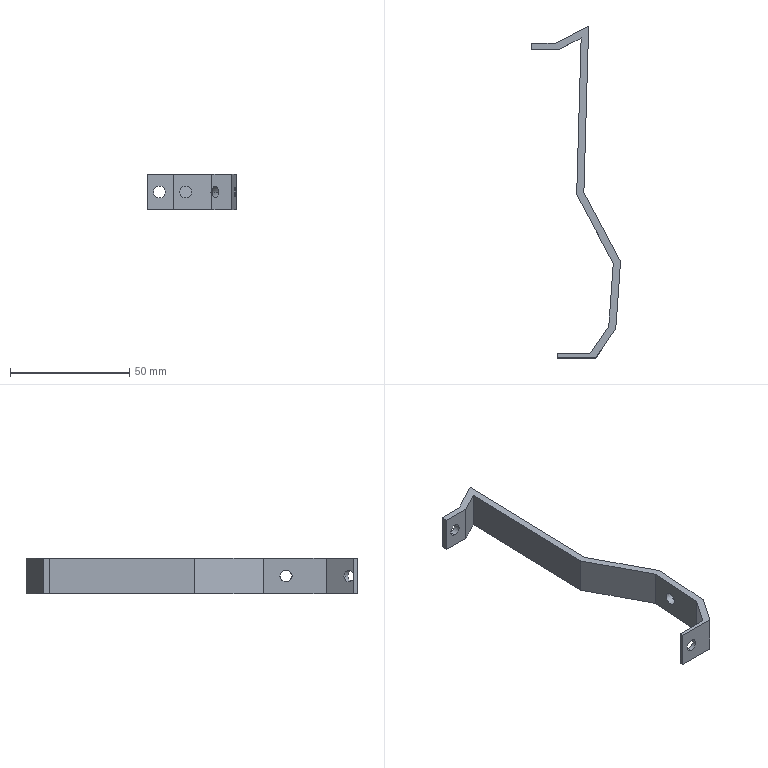Part | SolidWorks | features ICE 4, Extrusion 1, RevCut 1 | 1 solid | 26 faces | box 37.394 x 139.343 x 15 mm | volume 7600 mm3 | plane 18 | torus 4 | cylinder 4 | commonest cylinder face diameters 5 x4
STEP:
#1=CARTESIAN_POINT('',(17.078,-131.945,0.));
#2=VERTEX_POINT('',#1);
#3=CARTESIAN_POINT('',(19.895,-127.783,0.));
#4=VERTEX_POINT('',#3);
#5=CARTESIAN_POINT('',(17.078,-131.945,0.));
#6=CARTESIAN_POINT('',(17.078,-131.945,0.1641));
#7=CARTESIAN_POINT('',(17.087,-131.932,0.3266));
#8=CARTESIAN_POINT('',(17.123,-131.879,0.6485));
#9=CARTESIAN_POINT('',(17.15,-131.838,0.8079));
#10=CARTESIAN_POINT('',(17.256,-131.682,1.26));
#11=CARTESIAN_POINT('',(17.361,-131.527,1.54));
#12=CARTESIAN_POINT('',(17.556,-131.239,1.885));
#13=CARTESIAN_POINT('',(17.628,-131.132,1.99));
#14=CARTESIAN_POINT('',(17.782,-130.905,2.172));
#15=CARTESIAN_POINT('',(17.863,-130.785,2.248));
#16=CARTESIAN_POINT('',(18.033,-130.535,2.373));
#17=CARTESIAN_POINT('',(18.122,-130.402,2.421));
#18=CARTESIAN_POINT('',(18.302,-130.136,2.484));
#19=CARTESIAN_POINT('',(18.393,-130.002,2.5));
#20=CARTESIAN_POINT('',(18.578,-129.729,2.5));
#21=CARTESIAN_POINT('',(18.67,-129.592,2.484));
#22=CARTESIAN_POINT('',(18.85,-129.327,2.42));
#23=CARTESIAN_POINT('',(18.938,-129.196,2.373));
#24=CARTESIAN_POINT('',(19.11,-128.943,2.247));
#25=CARTESIAN_POINT('',(19.19,-128.824,2.17));
#26=CARTESIAN_POINT('',(19.343,-128.598,1.99));
#27=CARTESIAN_POINT('',(19.416,-128.491,1.885));
#28=CARTESIAN_POINT('',(19.546,-128.298,1.653));
#29=CARTESIAN_POINT('',(19.605,-128.212,1.528));
#30=CARTESIAN_POINT('',(19.707,-128.06,1.256));
#31=CARTESIAN_POINT('',(19.752,-127.994,1.109));
#32=CARTESIAN_POINT('',(19.858,-127.838,0.6566));
#33=CARTESIAN_POINT('',(19.895,-127.783,0.3266));
#34=CARTESIAN_POINT('',(19.895,-127.783,0.));
#35=B_SPLINE_CURVE_WITH_KNOTS('',3,(#5,#6,#7,#8,#9,#10,#11,#12,#13,#14,#15,#16,#17,#18,#19,#20,#21,#22,#23,#24,#25,#26,#27,#28,#29,#30,#31,#32,#33,#34),.UNSPECIFIED.,.F.,.F.,(4,2,2,2,2,2,2,2,2,2,2,2,2,2,4),(0.001854,0.002344,0.002834,0.003814,0.004304,0.004794,0.005284,0.005774,0.006263,0.006753,0.007243,0.007733,0.008223,0.008713,0.009693),.UNSPECIFIED.);
#36=EDGE_CURVE('',#2,#4,#35,.T.);
#37=ORIENTED_EDGE('',*,*,#36,.F.);
#38=CARTESIAN_POINT('',(14.593,-130.264,0.));
#39=VERTEX_POINT('',#38);
#40=CARTESIAN_POINT('',(25.607,-116.664,0.));
#41=DIRECTION('',(0.,0.,-1.));
#42=DIRECTION('',(-1.,0.,0.));
#43=AXIS2_PLACEMENT_3D('',#40,#41,#42);
#44=CIRCLE('',#43,17.5);
#45=EDGE_CURVE('',#2,#39,#44,.T.);
#46=ORIENTED_EDGE('',*,*,#45,.T.);
#47=CARTESIAN_POINT('',(17.41,-126.101,0.));
#48=VERTEX_POINT('',#47);
#49=CARTESIAN_POINT('',(17.41,-126.101,0.));
#50=CARTESIAN_POINT('',(17.41,-126.101,0.1645));
#51=CARTESIAN_POINT('',(17.401,-126.115,0.3271));
#52=CARTESIAN_POINT('',(17.365,-126.168,0.6482));
#53=CARTESIAN_POINT('',(17.338,-126.209,0.8078));
#54=CARTESIAN_POINT('',(17.267,-126.313,1.11));
#55=CARTESIAN_POINT('',(17.223,-126.377,1.254));
#56=CARTESIAN_POINT('',(17.12,-126.53,1.527));
#57=CARTESIAN_POINT('',(17.061,-126.617,1.654));
#58=CARTESIAN_POINT('',(16.866,-126.905,1.999));
#59=CARTESIAN_POINT('',(16.709,-127.138,2.185));
#60=CARTESIAN_POINT('',(16.455,-127.513,2.372));
#61=CARTESIAN_POINT('',(16.365,-127.645,2.42));
#62=CARTESIAN_POINT('',(16.185,-127.912,2.484));
#63=CARTESIAN_POINT('',(16.094,-128.046,2.5));
#64=CARTESIAN_POINT('',(15.91,-128.318,2.5));
#65=CARTESIAN_POINT('',(15.817,-128.456,2.484));
#66=CARTESIAN_POINT('',(15.637,-128.721,2.421));
#67=CARTESIAN_POINT('',(15.55,-128.851,2.374));
#68=CARTESIAN_POINT('',(15.378,-129.104,2.248));
#69=CARTESIAN_POINT('',(15.297,-129.224,2.171));
#70=CARTESIAN_POINT('',(15.144,-129.45,1.991));
#71=CARTESIAN_POINT('',(15.072,-129.556,1.886));
#72=CARTESIAN_POINT('',(14.941,-129.75,1.654));
#73=CARTESIAN_POINT('',(14.883,-129.836,1.528));
#74=CARTESIAN_POINT('',(14.781,-129.987,1.257));
#75=CARTESIAN_POINT('',(14.736,-130.053,1.11));
#76=CARTESIAN_POINT('',(14.666,-130.157,0.8073));
#77=CARTESIAN_POINT('',(14.639,-130.197,0.6512));
#78=CARTESIAN_POINT('',(14.603,-130.25,0.3285));
#79=CARTESIAN_POINT('',(14.593,-130.264,0.1633));
#80=CARTESIAN_POINT('',(14.593,-130.264,0.));
#81=B_SPLINE_CURVE_WITH_KNOTS('',3,(#49,#50,#51,#52,#53,#54,#55,#56,#57,#58,#59,#60,#61,#62,#63,#64,#65,#66,#67,#68,#69,#70,#71,#72,#73,#74,#75,#76,#77,#78,#79,#80),.UNSPECIFIED.,.F.,.F.,(4,2,2,2,2,2,2,2,2,2,2,2,2,2,2,4),(0.006023,0.006513,0.007003,0.007492,0.007982,0.008962,0.009452,0.009942,0.01043,0.01092,0.01141,0.0119,0.01239,0.01288,0.01337,0.01386),.UNSPECIFIED.);
#82=EDGE_CURVE('',#48,#39,#81,.T.);
#83=ORIENTED_EDGE('',*,*,#82,.F.);
#84=CARTESIAN_POINT('',(25.607,-116.664,0.));
#85=DIRECTION('',(0.,0.,-1.));
#86=DIRECTION('',(-1.,0.,0.));
#87=AXIS2_PLACEMENT_3D('',#84,#85,#86);
#88=CIRCLE('',#87,12.5);
#89=EDGE_CURVE('',#4,#48,#88,.T.);
#90=ORIENTED_EDGE('',*,*,#89,.F.);
#91=EDGE_LOOP('',(#37,#46,#83,#90));
#92=FACE_OUTER_BOUND('',#91,.T.);
#93=CARTESIAN_POINT('',(25.607,-116.664,0.));
#94=DIRECTION('',(0.,0.,-1.));
#95=DIRECTION('',(-1.,0.,0.));
#96=AXIS2_PLACEMENT_3D('',#93,#94,#95);
#97=TOROIDAL_SURFACE('',#96,15.,2.5);
#98=ADVANCED_FACE('',(#92),#97,.F.);
#99=CARTESIAN_POINT('',(23.843,-99.253,0.));
#100=VERTEX_POINT('',#99);
#101=CARTESIAN_POINT('',(23.479,-104.347,0.));
#102=VERTEX_POINT('',#101);
#103=CARTESIAN_POINT('',(23.843,-99.253,0.));
#104=CARTESIAN_POINT('',(23.843,-99.253,0.1653));
#105=CARTESIAN_POINT('',(23.842,-99.27,0.3291));
#106=CARTESIAN_POINT('',(23.837,-99.336,0.6537));
#107=CARTESIAN_POINT('',(23.834,-99.386,0.8139));
#108=CARTESIAN_POINT('',(23.82,-99.578,1.269));
#109=CARTESIAN_POINT('',(23.806,-99.77,1.548));
#110=CARTESIAN_POINT('',(23.781,-100.124,1.893));
#111=CARTESIAN_POINT('',(23.772,-100.255,1.998));
#112=CARTESIAN_POINT('',(23.752,-100.532,2.178));
#113=CARTESIAN_POINT('',(23.742,-100.678,2.253));
#114=CARTESIAN_POINT('',(23.72,-100.984,2.376));
#115=CARTESIAN_POINT('',(23.708,-101.145,2.423));
#116=CARTESIAN_POINT('',(23.685,-101.468,2.485));
#117=CARTESIAN_POINT('',(23.673,-101.631,2.5));
#118=CARTESIAN_POINT('',(23.638,-102.13,2.499));
#119=CARTESIAN_POINT('',(23.614,-102.456,2.435));
#120=CARTESIAN_POINT('',(23.582,-102.917,2.249));
#121=CARTESIAN_POINT('',(23.571,-103.063,2.173));
#122=CARTESIAN_POINT('',(23.551,-103.339,1.994));
#123=CARTESIAN_POINT('',(23.542,-103.47,1.889));
#124=CARTESIAN_POINT('',(23.525,-103.707,1.66));
#125=CARTESIAN_POINT('',(23.517,-103.814,1.534));
#126=CARTESIAN_POINT('',(23.504,-104.002,1.263));
#127=CARTESIAN_POINT('',(23.498,-104.083,1.116));
#128=CARTESIAN_POINT('',(23.489,-104.213,0.813));
#129=CARTESIAN_POINT('',(23.485,-104.263,0.656));
#130=CARTESIAN_POINT('',(23.481,-104.33,0.33));
#131=CARTESIAN_POINT('',(23.479,-104.347,0.1646));
#132=CARTESIAN_POINT('',(23.479,-104.347,0.));
#133=B_SPLINE_CURVE_WITH_KNOTS('',3,(#103,#104,#105,#106,#107,#108,#109,#110,#111,#112,#113,#114,#115,#116,#117,#118,#119,#120,#121,#122,#123,#124,#125,#126,#127,#128,#129,#130,#131,#132),.UNSPECIFIED.,.F.,.F.,(4,2,2,2,2,2,2,2,2,2,2,2,2,2,4),(0.007039,0.007533,0.008027,0.009014,0.009508,0.01,0.0105,0.01099,0.01198,0.01247,0.01296,0.01346,0.01395,0.01445,0.01494),.UNSPECIFIED.);
#134=EDGE_CURVE('',#100,#102,#133,.T.);
#135=ORIENTED_EDGE('',*,*,#134,.F.);
#136=CARTESIAN_POINT('',(26.854,-99.209,0.));
#137=VERTEX_POINT('',#136);
#138=CARTESIAN_POINT('',(25.607,-116.664,0.));
#139=DIRECTION('',(0.,0.,-1.));
#140=DIRECTION('',(-1.,0.,0.));
#141=AXIS2_PLACEMENT_3D('',#138,#139,#140);
#142=CIRCLE('',#141,17.5);
#143=EDGE_CURVE('',#100,#137,#142,.T.);
#144=ORIENTED_EDGE('',*,*,#143,.T.);
#145=CARTESIAN_POINT('',(26.498,-104.196,0.));
#146=VERTEX_POINT('',#145);
#147=CARTESIAN_POINT('',(26.676,-101.702,0.));
#148=DIRECTION('',(-0.9975,0.07125,0.));
#149=DIRECTION('',(-0.07125,-0.9975,0.));
#150=AXIS2_PLACEMENT_3D('',#147,#148,#149);
#151=CIRCLE('',#150,2.5);
#152=EDGE_CURVE('',#146,#137,#151,.T.);
#153=ORIENTED_EDGE('',*,*,#152,.F.);
#154=CARTESIAN_POINT('',(25.607,-116.664,0.));
#155=DIRECTION('',(0.,0.,-1.));
#156=DIRECTION('',(-1.,0.,0.));
#157=AXIS2_PLACEMENT_3D('',#154,#155,#156);
#158=CIRCLE('',#157,12.5);
#159=EDGE_CURVE('',#102,#146,#158,.T.);
#160=ORIENTED_EDGE('',*,*,#159,.F.);
#161=EDGE_LOOP('',(#135,#144,#153,#160));
#162=FACE_OUTER_BOUND('',#161,.T.);
#163=CARTESIAN_POINT('',(25.607,-116.664,0.));
#164=DIRECTION('',(0.,0.,-1.));
#165=DIRECTION('',(-1.,0.,0.));
#166=AXIS2_PLACEMENT_3D('',#163,#164,#165);
#167=TOROIDAL_SURFACE('',#166,15.,2.5);
#168=ADVANCED_FACE('',(#162),#167,.F.);
#169=CARTESIAN_POINT('',(6.,-130.319,-2.5));
#170=VERTEX_POINT('',#169);
#171=CARTESIAN_POINT('',(6.,-130.319,2.5));
#172=VERTEX_POINT('',#171);
#173=CARTESIAN_POINT('',(6.,-130.319,0.));
#174=DIRECTION('',(0.,1.,0.));
#175=DIRECTION('',(0.,0.,1.));
#176=AXIS2_PLACEMENT_3D('',#173,#174,#175);
#177=CIRCLE('',#176,2.5);
#178=EDGE_CURVE('',#170,#172,#177,.T.);
#179=ORIENTED_EDGE('',*,*,#178,.T.);
#180=CARTESIAN_POINT('',(6.,-132.,2.5));
#181=VERTEX_POINT('',#180);
#182=CARTESIAN_POINT('',(6.,-122.,2.5));
#183=DIRECTION('',(0.,-1.,0.));
#184=VECTOR('',#183,1000.);
#185=LINE('',#182,#184);
#186=EDGE_CURVE('',#172,#181,#185,.T.);
#187=ORIENTED_EDGE('',*,*,#186,.T.);
#188=CARTESIAN_POINT('',(6.,-132.,-2.5));
#189=VERTEX_POINT('',#188);
#190=CARTESIAN_POINT('',(6.,-132.,0.));
#191=DIRECTION('',(0.,-1.,0.));
#192=DIRECTION('',(0.,0.,-1.));
#193=AXIS2_PLACEMENT_3D('',#190,#191,#192);
#194=CIRCLE('',#193,2.5);
#195=EDGE_CURVE('',#181,#189,#194,.T.);
#196=ORIENTED_EDGE('',*,*,#195,.T.);
#197=CARTESIAN_POINT('',(6.,-122.,-2.5));
#198=DIRECTION('',(0.,-1.,0.));
#199=VECTOR('',#198,1000.);
#200=LINE('',#197,#199);
#201=EDGE_CURVE('',#170,#189,#200,.T.);
#202=ORIENTED_EDGE('',*,*,#201,.F.);
#203=EDGE_LOOP('',(#179,#187,#196,#202));
#204=FACE_OUTER_BOUND('',#203,.T.);
#205=CARTESIAN_POINT('',(6.,-122.,0.));
#206=DIRECTION('',(0.,-1.,0.));
#207=DIRECTION('',(0.,0.,-1.));
#208=AXIS2_PLACEMENT_3D('',#205,#206,#207);
#209=CYLINDRICAL_SURFACE('',#208,2.5);
#210=ADVANCED_FACE('',(#204),#209,.F.);
#211=CARTESIAN_POINT('',(-5.,-2.657,2.5));
#212=VERTEX_POINT('',#211);
#213=CARTESIAN_POINT('',(-5.,-2.657,-2.5));
#214=VERTEX_POINT('',#213);
#215=CARTESIAN_POINT('',(-5.,-2.657,0.));
#216=DIRECTION('',(0.,-1.,0.));
#217=DIRECTION('',(0.,0.,-1.));
#218=AXIS2_PLACEMENT_3D('',#215,#216,#217);
#219=CIRCLE('',#218,2.5);
#220=EDGE_CURVE('',#212,#214,#219,.T.);
#221=ORIENTED_EDGE('',*,*,#220,.T.);
#222=CARTESIAN_POINT('',(-5.,0.,-2.5));
#223=VERTEX_POINT('',#222);
#224=CARTESIAN_POINT('',(-5.,-5.,-2.5));
#225=DIRECTION('',(0.,1.,0.));
#226=VECTOR('',#225,1000.);
#227=LINE('',#224,#226);
#228=EDGE_CURVE('',#214,#223,#227,.T.);
#229=ORIENTED_EDGE('',*,*,#228,.T.);
#230=CARTESIAN_POINT('',(-5.,0.,2.5));
#231=VERTEX_POINT('',#230);
#232=CARTESIAN_POINT('',(-5.,0.,0.));
#233=DIRECTION('',(0.,1.,0.));
#234=DIRECTION('',(0.,0.,1.));
#235=AXIS2_PLACEMENT_3D('',#232,#233,#234);
#236=CIRCLE('',#235,2.5);
#237=EDGE_CURVE('',#223,#231,#236,.T.);
#238=ORIENTED_EDGE('',*,*,#237,.T.);
#239=CARTESIAN_POINT('',(-5.,-5.,2.5));
#240=DIRECTION('',(0.,1.,0.));
#241=VECTOR('',#240,1000.);
#242=LINE('',#239,#241);
#243=EDGE_CURVE('',#212,#231,#242,.T.);
#244=ORIENTED_EDGE('',*,*,#243,.F.);
#245=EDGE_LOOP('',(#221,#229,#238,#244));
#246=FACE_OUTER_BOUND('',#245,.T.);
#247=CARTESIAN_POINT('',(-5.,-5.,0.));
#248=DIRECTION('',(0.,1.,0.));
#249=DIRECTION('',(0.,0.,1.));
#250=AXIS2_PLACEMENT_3D('',#247,#248,#249);
#251=CYLINDRICAL_SURFACE('',#250,2.5);
#252=ADVANCED_FACE('',(#246),#251,.F.);
#253=CARTESIAN_POINT('',(1.394,-2.657,-7.5));
#254=VERTEX_POINT('',#253);
#255=CARTESIAN_POINT('',(10.855,2.306,-7.5));
#256=VERTEX_POINT('',#255);
#257=CARTESIAN_POINT('',(1.394,-2.657,-7.5));
#258=DIRECTION('',(0.8856,0.4645,0.));
#259=VECTOR('',#258,1000.);
#260=LINE('',#257,#259);
#261=EDGE_CURVE('',#254,#256,#260,.T.);
#262=ORIENTED_EDGE('',*,*,#261,.T.);
#263=CARTESIAN_POINT('',(10.855,2.306,7.5));
#264=VERTEX_POINT('',#263);
#265=CARTESIAN_POINT('',(10.855,2.306,7.5));
#266=DIRECTION('',(0.,0.,-1.));
#267=VECTOR('',#266,1000.);
#268=LINE('',#265,#267);
#269=EDGE_CURVE('',#264,#256,#268,.T.);
#270=ORIENTED_EDGE('',*,*,#269,.F.);
#271=CARTESIAN_POINT('',(1.394,-2.657,7.5));
#272=VERTEX_POINT('',#271);
#273=CARTESIAN_POINT('',(1.394,-2.657,7.5));
#274=DIRECTION('',(0.8856,0.4645,0.));
#275=VECTOR('',#274,1000.);
#276=LINE('',#273,#275);
#277=EDGE_CURVE('',#272,#264,#276,.T.);
#278=ORIENTED_EDGE('',*,*,#277,.F.);
#279=CARTESIAN_POINT('',(1.394,-2.657,7.5));
#280=DIRECTION('',(0.,0.,-1.));
#281=VECTOR('',#280,1000.);
#282=LINE('',#279,#281);
#283=EDGE_CURVE('',#272,#254,#282,.T.);
#284=ORIENTED_EDGE('',*,*,#283,.T.);
#285=EDGE_LOOP('',(#262,#270,#278,#284));
#286=FACE_OUTER_BOUND('',#285,.T.);
#287=CARTESIAN_POINT('',(1.394,-2.657,7.5));
#288=DIRECTION('',(-0.4645,0.8856,0.));
#289=DIRECTION('',(-0.8856,-0.4645,0.));
#290=AXIS2_PLACEMENT_3D('',#287,#288,#289);
#291=PLANE('',#290);
#292=ADVANCED_FACE('',(#286),#291,.F.);
#293=CARTESIAN_POINT('',(8.979,-63.363,-7.5));
#294=VERTEX_POINT('',#293);
#295=CARTESIAN_POINT('',(10.855,2.306,-7.5));
#296=DIRECTION('',(-0.02856,-0.9996,0.));
#297=VECTOR('',#296,1000.);
#298=LINE('',#295,#297);
#299=EDGE_CURVE('',#256,#294,#298,.T.);
#300=ORIENTED_EDGE('',*,*,#299,.T.);
#301=CARTESIAN_POINT('',(8.979,-63.363,7.5));
#302=VERTEX_POINT('',#301);
#303=CARTESIAN_POINT('',(8.979,-63.363,7.5));
#304=DIRECTION('',(0.,0.,-1.));
#305=VECTOR('',#304,1000.);
#306=LINE('',#303,#305);
#307=EDGE_CURVE('',#302,#294,#306,.T.);
#308=ORIENTED_EDGE('',*,*,#307,.F.);
#309=CARTESIAN_POINT('',(10.855,2.306,7.5));
#310=DIRECTION('',(-0.02856,-0.9996,0.));
#311=VECTOR('',#310,1000.);
#312=LINE('',#309,#311);
#313=EDGE_CURVE('',#264,#302,#312,.T.);
#314=ORIENTED_EDGE('',*,*,#313,.F.);
#315=ORIENTED_EDGE('',*,*,#269,.T.);
#316=EDGE_LOOP('',(#300,#308,#314,#315));
#317=FACE_OUTER_BOUND('',#316,.T.);
#318=CARTESIAN_POINT('',(10.855,2.306,7.5));
#319=DIRECTION('',(0.9996,-0.02856,0.));
#320=DIRECTION('',(0.02856,0.9996,0.));
#321=AXIS2_PLACEMENT_3D('',#318,#319,#320);
#322=PLANE('',#321);
#323=ADVANCED_FACE('',(#317),#322,.F.);
#324=CARTESIAN_POINT('',(24.34,-92.302,-7.5));
#325=VERTEX_POINT('',#324);
#326=CARTESIAN_POINT('',(8.979,-63.363,-7.5));
#327=DIRECTION('',(0.4689,-0.8833,0.));
#328=VECTOR('',#327,1000.);
#329=LINE('',#326,#328);
#330=EDGE_CURVE('',#294,#325,#329,.T.);
#331=ORIENTED_EDGE('',*,*,#330,.T.);
#332=CARTESIAN_POINT('',(24.34,-92.302,7.5));
#333=VERTEX_POINT('',#332);
#334=CARTESIAN_POINT('',(24.34,-92.302,7.5));
#335=DIRECTION('',(0.,0.,-1.));
#336=VECTOR('',#335,1000.);
#337=LINE('',#334,#336);
#338=EDGE_CURVE('',#333,#325,#337,.T.);
#339=ORIENTED_EDGE('',*,*,#338,.F.);
#340=CARTESIAN_POINT('',(8.979,-63.363,7.5));
#341=DIRECTION('',(0.4689,-0.8833,0.));
#342=VECTOR('',#341,1000.);
#343=LINE('',#340,#342);
#344=EDGE_CURVE('',#302,#333,#343,.T.);
#345=ORIENTED_EDGE('',*,*,#344,.F.);
#346=ORIENTED_EDGE('',*,*,#307,.T.);
#347=EDGE_LOOP('',(#331,#339,#345,#346));
#348=FACE_OUTER_BOUND('',#347,.T.);
#349=CARTESIAN_POINT('',(8.979,-63.363,7.5));
#350=DIRECTION('',(0.8833,0.4689,0.));
#351=DIRECTION('',(-0.4689,0.8833,0.));
#352=AXIS2_PLACEMENT_3D('',#349,#350,#351);
#353=PLANE('',#352);
#354=ADVANCED_FACE('',(#348),#353,.F.);
#355=CARTESIAN_POINT('',(23.479,-104.347,0.));
#356=CARTESIAN_POINT('',(23.479,-104.347,-0.329));
#357=CARTESIAN_POINT('',(23.484,-104.277,-0.6643));
#358=CARTESIAN_POINT('',(23.498,-104.081,-1.12));
#359=CARTESIAN_POINT('',(23.504,-104.001,-1.264));
#360=CARTESIAN_POINT('',(23.518,-103.813,-1.535));
#361=CARTESIAN_POINT('',(23.525,-103.704,-1.663));
#362=CARTESIAN_POINT('',(23.542,-103.467,-1.892));
#363=CARTESIAN_POINT('',(23.551,-103.339,-1.994));
#364=CARTESIAN_POINT('',(23.571,-103.06,-2.174));
#365=CARTESIAN_POINT('',(23.582,-102.913,-2.251));
#366=CARTESIAN_POINT('',(23.614,-102.456,-2.435));
#367=CARTESIAN_POINT('',(23.638,-102.124,-2.499));
#368=CARTESIAN_POINT('',(23.673,-101.632,-2.5));
#369=CARTESIAN_POINT('',(23.685,-101.465,-2.485));
#370=CARTESIAN_POINT('',(23.708,-101.141,-2.422));
#371=CARTESIAN_POINT('',(23.72,-100.984,-2.376));
#372=CARTESIAN_POINT('',(23.741,-100.678,-2.253));
#373=CARTESIAN_POINT('',(23.752,-100.529,-2.176));
#374=CARTESIAN_POINT('',(23.772,-100.253,-1.997));
#375=CARTESIAN_POINT('',(23.781,-100.125,-1.894));
#376=CARTESIAN_POINT('',(23.806,-99.769,-1.547));
#377=CARTESIAN_POINT('',(23.82,-99.58,-1.272));
#378=CARTESIAN_POINT('',(23.834,-99.385,-0.8125));
#379=CARTESIAN_POINT('',(23.837,-99.336,-0.6552));
#380=CARTESIAN_POINT('',(23.842,-99.27,-0.3325));
#381=CARTESIAN_POINT('',(23.843,-99.253,-0.1652));
#382=CARTESIAN_POINT('',(23.843,-99.253,0.));
#383=B_SPLINE_CURVE_WITH_KNOTS('',3,(#355,#356,#357,#358,#359,#360,#361,#362,#363,#364,#365,#366,#367,#368,#369,#370,#371,#372,#373,#374,#375,#376,#377,#378,#379,#380,#381,#382),.UNSPECIFIED.,.F.,.F.,(4,2,2,2,2,2,2,2,2,2,2,2,2,4),(0.01494,0.01593,0.01642,0.01691,0.01741,0.0179,0.01889,0.01938,0.01987,0.02037,0.02086,0.02185,0.02234,0.02283),.UNSPECIFIED.);
#384=EDGE_CURVE('',#102,#100,#383,.T.);
#385=ORIENTED_EDGE('',*,*,#384,.T.);
#386=ORIENTED_EDGE('',*,*,#134,.T.);
#387=EDGE_LOOP('',(#385,#386));
#388=FACE_BOUND('',#387,.T.);
#389=CARTESIAN_POINT('',(22.458,-118.641,-7.5));
#390=VERTEX_POINT('',#389);
#391=CARTESIAN_POINT('',(24.34,-92.302,-7.5));
#392=DIRECTION('',(-0.07125,-0.9975,0.));
#393=VECTOR('',#392,1000.);
#394=LINE('',#391,#393);
#395=EDGE_CURVE('',#325,#390,#394,.T.);
#396=ORIENTED_EDGE('',*,*,#395,.T.);
#397=CARTESIAN_POINT('',(22.458,-118.641,7.5));
#398=VERTEX_POINT('',#397);
#399=CARTESIAN_POINT('',(22.458,-118.641,7.5));
#400=DIRECTION('',(0.,0.,-1.));
#401=VECTOR('',#400,1000.);
#402=LINE('',#399,#401);
#403=EDGE_CURVE('',#398,#390,#402,.T.);
#404=ORIENTED_EDGE('',*,*,#403,.F.);
#405=CARTESIAN_POINT('',(24.34,-92.302,7.5));
#406=DIRECTION('',(-0.07125,-0.9975,0.));
#407=VECTOR('',#406,1000.);
#408=LINE('',#405,#407);
#409=EDGE_CURVE('',#333,#398,#408,.T.);
#410=ORIENTED_EDGE('',*,*,#409,.F.);
#411=ORIENTED_EDGE('',*,*,#338,.T.);
#412=EDGE_LOOP('',(#396,#404,#410,#411));
#413=FACE_OUTER_BOUND('',#412,.T.);
#414=CARTESIAN_POINT('',(24.34,-92.302,7.5));
#415=DIRECTION('',(0.9975,-0.07125,0.));
#416=DIRECTION('',(0.07125,0.9975,0.));
#417=AXIS2_PLACEMENT_3D('',#414,#415,#416);
#418=PLANE('',#417);
#419=ADVANCED_FACE('',(#388,#413),#418,.F.);
#420=ORIENTED_EDGE('',*,*,#82,.T.);
#421=CARTESIAN_POINT('',(14.593,-130.264,0.));
#422=CARTESIAN_POINT('',(14.593,-130.264,-0.3265));
#423=CARTESIAN_POINT('',(14.63,-130.209,-0.6563));
#424=CARTESIAN_POINT('',(14.771,-130.001,-1.26));
#425=CARTESIAN_POINT('',(14.877,-129.844,-1.541));
#426=CARTESIAN_POINT('',(15.073,-129.555,-1.888));
#427=CARTESIAN_POINT('',(15.144,-129.45,-1.991));
#428=CARTESIAN_POINT('',(15.297,-129.224,-2.172));
#429=CARTESIAN_POINT('',(15.38,-129.102,-2.25));
#430=CARTESIAN_POINT('',(15.55,-128.851,-2.374));
#431=CARTESIAN_POINT('',(15.637,-128.721,-2.421));
#432=CARTESIAN_POINT('',(15.819,-128.454,-2.484));
#433=CARTESIAN_POINT('',(15.911,-128.317,-2.5));
#434=CARTESIAN_POINT('',(16.094,-128.047,-2.5));
#435=CARTESIAN_POINT('',(16.186,-127.911,-2.484));
#436=CARTESIAN_POINT('',(16.367,-127.643,-2.42));
#437=CARTESIAN_POINT('',(16.455,-127.514,-2.372));
#438=CARTESIAN_POINT('',(16.624,-127.263,-2.248));
#439=CARTESIAN_POINT('',(16.706,-127.141,-2.17));
#440=CARTESIAN_POINT('',(16.86,-126.915,-1.988));
#441=CARTESIAN_POINT('',(16.93,-126.81,-1.885));
#442=CARTESIAN_POINT('',(17.061,-126.617,-1.654));
#443=CARTESIAN_POINT('',(17.121,-126.529,-1.526));
#444=CARTESIAN_POINT('',(17.223,-126.378,-1.255));
#445=CARTESIAN_POINT('',(17.266,-126.314,-1.112));
#446=CARTESIAN_POINT('',(17.338,-126.208,-0.8067));
#447=CARTESIAN_POINT('',(17.365,-126.168,-0.6496));
#448=CARTESIAN_POINT('',(17.401,-126.115,-0.3296));
#449=CARTESIAN_POINT('',(17.41,-126.101,-0.1645));
#450=CARTESIAN_POINT('',(17.41,-126.101,0.));
#451=B_SPLINE_CURVE_WITH_KNOTS('',3,(#421,#422,#423,#424,#425,#426,#427,#428,#429,#430,#431,#432,#433,#434,#435,#436,#437,#438,#439,#440,#441,#442,#443,#444,#445,#446,#447,#448,#449,#450),.UNSPECIFIED.,.F.,.F.,(4,2,2,2,2,2,2,2,2,2,2,2,2,2,4),(0.01386,0.01484,0.01582,0.01631,0.0168,0.01729,0.01778,0.01827,0.01876,0.01925,0.01973,0.02022,0.02071,0.0212,0.02169),.UNSPECIFIED.);
#452=EDGE_CURVE('',#39,#48,#451,.T.);
#453=ORIENTED_EDGE('',*,*,#452,.T.);
#454=EDGE_LOOP('',(#420,#453));
#455=FACE_BOUND('',#454,.T.);
#456=CARTESIAN_POINT('',(14.556,-130.319,-7.5));
#457=VERTEX_POINT('',#456);
#458=CARTESIAN_POINT('',(22.458,-118.641,-7.5));
#459=DIRECTION('',(-0.5604,-0.8282,0.));
#460=VECTOR('',#459,1000.);
#461=LINE('',#458,#460);
#462=EDGE_CURVE('',#390,#457,#461,.T.);
#463=ORIENTED_EDGE('',*,*,#462,.T.);
#464=CARTESIAN_POINT('',(14.556,-130.319,7.5));
#465=VERTEX_POINT('',#464);
#466=CARTESIAN_POINT('',(14.556,-130.319,7.5));
#467=DIRECTION('',(0.,0.,-1.));
#468=VECTOR('',#467,1000.);
#469=LINE('',#466,#468);
#470=EDGE_CURVE('',#465,#457,#469,.T.);
#471=ORIENTED_EDGE('',*,*,#470,.F.);
#472=CARTESIAN_POINT('',(22.458,-118.641,7.5));
#473=DIRECTION('',(-0.5604,-0.8282,0.));
#474=VECTOR('',#473,1000.);
#475=LINE('',#472,#474);
#476=EDGE_CURVE('',#398,#465,#475,.T.);
#477=ORIENTED_EDGE('',*,*,#476,.F.);
#478=ORIENTED_EDGE('',*,*,#403,.T.);
#479=EDGE_LOOP('',(#463,#471,#477,#478));
#480=FACE_OUTER_BOUND('',#479,.T.);
#481=CARTESIAN_POINT('',(22.458,-118.641,7.5));
#482=DIRECTION('',(0.8282,-0.5604,0.));
#483=DIRECTION('',(0.5604,0.8282,0.));
#484=AXIS2_PLACEMENT_3D('',#481,#482,#483);
#485=PLANE('',#484);
#486=ADVANCED_FACE('',(#455,#480),#485,.F.);
#487=CARTESIAN_POINT('',(19.895,-127.783,0.));
#488=CARTESIAN_POINT('',(19.895,-127.783,-0.1632));
#489=CARTESIAN_POINT('',(19.886,-127.796,-0.328));
#490=CARTESIAN_POINT('',(19.849,-127.85,-0.6508));
#491=CARTESIAN_POINT('',(19.822,-127.89,-0.8069));
#492=CARTESIAN_POINT('',(19.752,-127.994,-1.109));
#493=CARTESIAN_POINT('',(19.707,-128.06,-1.256));
#494=CARTESIAN_POINT('',(19.605,-128.211,-1.527));
#495=CARTESIAN_POINT('',(19.547,-128.297,-1.653));
#496=CARTESIAN_POINT('',(19.416,-128.491,-1.884));
#497=CARTESIAN_POINT('',(19.344,-128.597,-1.989));
#498=CARTESIAN_POINT('',(19.191,-128.823,-2.17));
#499=CARTESIAN_POINT('',(19.11,-128.943,-2.247));
#500=CARTESIAN_POINT('',(18.939,-129.196,-2.373));
#501=CARTESIAN_POINT('',(18.851,-129.325,-2.42));
#502=CARTESIAN_POINT('',(18.671,-129.591,-2.483));
#503=CARTESIAN_POINT('',(18.578,-129.728,-2.5));
#504=CARTESIAN_POINT('',(18.395,-130.,-2.5));
#505=CARTESIAN_POINT('',(18.304,-130.134,-2.484));
#506=CARTESIAN_POINT('',(18.123,-130.4,-2.422));
#507=CARTESIAN_POINT('',(18.034,-130.533,-2.374));
#508=CARTESIAN_POINT('',(17.78,-130.908,-2.188));
#509=CARTESIAN_POINT('',(17.623,-131.14,-2.003));
#510=CARTESIAN_POINT('',(17.361,-131.528,-1.538));
#511=CARTESIAN_POINT('',(17.257,-131.681,-1.264));
#512=CARTESIAN_POINT('',(17.15,-131.839,-0.8064));
#513=CARTESIAN_POINT('',(17.123,-131.878,-0.6501));
#514=CARTESIAN_POINT('',(17.087,-131.931,-0.3298));
#515=CARTESIAN_POINT('',(17.078,-131.945,-0.164));
#516=CARTESIAN_POINT('',(17.078,-131.945,0.));
#517=B_SPLINE_CURVE_WITH_KNOTS('',3,(#487,#488,#489,#490,#491,#492,#493,#494,#495,#496,#497,#498,#499,#500,#501,#502,#503,#504,#505,#506,#507,#508,#509,#510,#511,#512,#513,#514,#515,#516),.UNSPECIFIED.,.F.,.F.,(4,2,2,2,2,2,2,2,2,2,2,2,2,2,4),(0.009693,0.01018,0.01067,0.01116,0.01165,0.01214,0.01263,0.01312,0.01361,0.0141,0.01459,0.01557,0.01655,0.01704,0.01753),.UNSPECIFIED.);
#518=EDGE_CURVE('',#4,#2,#517,.T.);
#519=ORIENTED_EDGE('',*,*,#518,.T.);
#520=ORIENTED_EDGE('',*,*,#36,.T.);
#521=EDGE_LOOP('',(#519,#520));
#522=FACE_BOUND('',#521,.T.);
#523=CARTESIAN_POINT('',(17.041,-132.,-7.5));
#524=VERTEX_POINT('',#523);
#525=CARTESIAN_POINT('',(25.394,-119.657,-7.5));
#526=VERTEX_POINT('',#525);
#527=CARTESIAN_POINT('',(25.394,-119.657,-7.5));
#528=DIRECTION('',(0.5604,0.8282,0.));
#529=VECTOR('',#528,1000.);
#530=LINE('',#527,#529);
#531=EDGE_CURVE('',#524,#526,#530,.T.);
#532=ORIENTED_EDGE('',*,*,#531,.T.);
#533=CARTESIAN_POINT('',(25.394,-119.657,7.5));
#534=VERTEX_POINT('',#533);
#535=CARTESIAN_POINT('',(25.394,-119.657,7.5));
#536=DIRECTION('',(0.,0.,-1.));
#537=VECTOR('',#536,1000.);
#538=LINE('',#535,#537);
#539=EDGE_CURVE('',#534,#526,#538,.T.);
#540=ORIENTED_EDGE('',*,*,#539,.F.);
#541=CARTESIAN_POINT('',(17.041,-132.,7.5));
#542=VERTEX_POINT('',#541);
#543=CARTESIAN_POINT('',(25.394,-119.657,7.5));
#544=DIRECTION('',(0.5604,0.8282,0.));
#545=VECTOR('',#544,1000.);
#546=LINE('',#543,#545);
#547=EDGE_CURVE('',#542,#534,#546,.T.);
#548=ORIENTED_EDGE('',*,*,#547,.F.);
#549=CARTESIAN_POINT('',(17.041,-132.,7.5));
#550=DIRECTION('',(0.,0.,-1.));
#551=VECTOR('',#550,1000.);
#552=LINE('',#549,#551);
#553=EDGE_CURVE('',#542,#524,#552,.T.);
#554=ORIENTED_EDGE('',*,*,#553,.T.);
#555=EDGE_LOOP('',(#532,#540,#548,#554));
#556=FACE_OUTER_BOUND('',#555,.T.);
#557=CARTESIAN_POINT('',(25.394,-119.657,7.5));
#558=DIRECTION('',(-0.8282,0.5604,0.));
#559=DIRECTION('',(-0.5604,-0.8282,0.));
#560=AXIS2_PLACEMENT_3D('',#557,#558,#559);
#561=PLANE('',#560);
#562=ADVANCED_FACE('',(#522,#556),#561,.F.);
#563=ORIENTED_EDGE('',*,*,#152,.T.);
#564=CARTESIAN_POINT('',(26.676,-101.702,0.));
#565=DIRECTION('',(-0.9975,0.07125,0.));
#566=DIRECTION('',(-0.07125,-0.9975,0.));
#567=AXIS2_PLACEMENT_3D('',#564,#565,#566);
#568=CIRCLE('',#567,2.5);
#569=EDGE_CURVE('',#137,#146,#568,.T.);
#570=ORIENTED_EDGE('',*,*,#569,.T.);
#571=EDGE_LOOP('',(#563,#570));
#572=FACE_BOUND('',#571,.T.);
#573=CARTESIAN_POINT('',(27.394,-91.657,-7.5));
#574=VERTEX_POINT('',#573);
#575=CARTESIAN_POINT('',(27.394,-91.657,-7.5));
#576=DIRECTION('',(0.07125,0.9975,0.));
#577=VECTOR('',#576,1000.);
#578=LINE('',#575,#577);
#579=EDGE_CURVE('',#526,#574,#578,.T.);
#580=ORIENTED_EDGE('',*,*,#579,.T.);
#581=CARTESIAN_POINT('',(27.394,-91.657,7.5));
#582=VERTEX_POINT('',#581);
#583=CARTESIAN_POINT('',(27.394,-91.657,7.5));
#584=DIRECTION('',(0.,0.,-1.));
#585=VECTOR('',#584,1000.);
#586=LINE('',#583,#585);
#587=EDGE_CURVE('',#582,#574,#586,.T.);
#588=ORIENTED_EDGE('',*,*,#587,.F.);
#589=CARTESIAN_POINT('',(27.394,-91.657,7.5));
#590=DIRECTION('',(0.07125,0.9975,0.));
#591=VECTOR('',#590,1000.);
#592=LINE('',#589,#591);
#593=EDGE_CURVE('',#534,#582,#592,.T.);
#594=ORIENTED_EDGE('',*,*,#593,.F.);
#595=ORIENTED_EDGE('',*,*,#539,.T.);
#596=EDGE_LOOP('',(#580,#588,#594,#595));
#597=FACE_OUTER_BOUND('',#596,.T.);
#598=CARTESIAN_POINT('',(27.394,-91.657,7.5));
#599=DIRECTION('',(-0.9975,0.07125,0.));
#600=DIRECTION('',(-0.07125,-0.9975,0.));
#601=AXIS2_PLACEMENT_3D('',#598,#599,#600);
#602=PLANE('',#601);
#603=ADVANCED_FACE('',(#572,#597),#602,.F.);
#604=CARTESIAN_POINT('',(12.,-62.657,-7.5));
#605=VERTEX_POINT('',#604);
#606=CARTESIAN_POINT('',(12.,-62.657,-7.5));
#607=DIRECTION('',(-0.4689,0.8833,0.));
#608=VECTOR('',#607,1000.);
#609=LINE('',#606,#608);
#610=EDGE_CURVE('',#574,#605,#609,.T.);
#611=ORIENTED_EDGE('',*,*,#610,.T.);
#612=CARTESIAN_POINT('',(12.,-62.657,7.5));
#613=VERTEX_POINT('',#612);
#614=CARTESIAN_POINT('',(12.,-62.657,7.5));
#615=DIRECTION('',(0.,0.,-1.));
#616=VECTOR('',#615,1000.);
#617=LINE('',#614,#616);
#618=EDGE_CURVE('',#613,#605,#617,.T.);
#619=ORIENTED_EDGE('',*,*,#618,.F.);
#620=CARTESIAN_POINT('',(12.,-62.657,7.5));
#621=DIRECTION('',(-0.4689,0.8833,0.));
#622=VECTOR('',#621,1000.);
#623=LINE('',#620,#622);
#624=EDGE_CURVE('',#582,#613,#623,.T.);
#625=ORIENTED_EDGE('',*,*,#624,.F.);
#626=ORIENTED_EDGE('',*,*,#587,.T.);
#627=EDGE_LOOP('',(#611,#619,#625,#626));
#628=FACE_OUTER_BOUND('',#627,.T.);
#629=CARTESIAN_POINT('',(12.,-62.657,7.5));
#630=DIRECTION('',(-0.8833,-0.4689,0.));
#631=DIRECTION('',(0.4689,-0.8833,0.));
#632=AXIS2_PLACEMENT_3D('',#629,#630,#631);
#633=PLANE('',#632);
#634=ADVANCED_FACE('',(#628),#633,.F.);
#635=CARTESIAN_POINT('',(14.,7.343,-7.5));
#636=VERTEX_POINT('',#635);
#637=CARTESIAN_POINT('',(14.,7.343,-7.5));
#638=DIRECTION('',(0.02856,0.9996,0.));
#639=VECTOR('',#638,1000.);
#640=LINE('',#637,#639);
#641=EDGE_CURVE('',#605,#636,#640,.T.);
#642=ORIENTED_EDGE('',*,*,#641,.T.);
#643=CARTESIAN_POINT('',(14.,7.343,7.5));
#644=VERTEX_POINT('',#643);
#645=CARTESIAN_POINT('',(14.,7.343,7.5));
#646=DIRECTION('',(0.,0.,-1.));
#647=VECTOR('',#646,1000.);
#648=LINE('',#645,#647);
#649=EDGE_CURVE('',#644,#636,#648,.T.);
#650=ORIENTED_EDGE('',*,*,#649,.F.);
#651=CARTESIAN_POINT('',(14.,7.343,7.5));
#652=DIRECTION('',(0.02856,0.9996,0.));
#653=VECTOR('',#652,1000.);
#654=LINE('',#651,#653);
#655=EDGE_CURVE('',#613,#644,#654,.T.);
#656=ORIENTED_EDGE('',*,*,#655,.F.);
#657=ORIENTED_EDGE('',*,*,#618,.T.);
#658=EDGE_LOOP('',(#642,#650,#656,#657));
#659=FACE_OUTER_BOUND('',#658,.T.);
#660=CARTESIAN_POINT('',(14.,7.343,7.5));
#661=DIRECTION('',(-0.9996,0.02856,0.));
#662=DIRECTION('',(-0.02856,-0.9996,0.));
#663=AXIS2_PLACEMENT_3D('',#660,#661,#662);
#664=PLANE('',#663);
#665=ADVANCED_FACE('',(#659),#664,.F.);
#666=CARTESIAN_POINT('',(0.,0.,-7.5));
#667=VERTEX_POINT('',#666);
#668=CARTESIAN_POINT('',(0.,0.,-7.5));
#669=DIRECTION('',(-0.8856,-0.4645,0.));
#670=VECTOR('',#669,1000.);
#671=LINE('',#668,#670);
#672=EDGE_CURVE('',#636,#667,#671,.T.);
#673=ORIENTED_EDGE('',*,*,#672,.T.);
#674=CARTESIAN_POINT('',(0.,0.,7.5));
#675=VERTEX_POINT('',#674);
#676=CARTESIAN_POINT('',(0.,0.,7.5));
#677=DIRECTION('',(0.,0.,-1.));
#678=VECTOR('',#677,1000.);
#679=LINE('',#676,#678);
#680=EDGE_CURVE('',#675,#667,#679,.T.);
#681=ORIENTED_EDGE('',*,*,#680,.F.);
#682=CARTESIAN_POINT('',(0.,0.,7.5));
#683=DIRECTION('',(-0.8856,-0.4645,0.));
#684=VECTOR('',#683,1000.);
#685=LINE('',#682,#684);
#686=EDGE_CURVE('',#644,#675,#685,.T.);
#687=ORIENTED_EDGE('',*,*,#686,.F.);
#688=ORIENTED_EDGE('',*,*,#649,.T.);
#689=EDGE_LOOP('',(#673,#681,#687,#688));
#690=FACE_OUTER_BOUND('',#689,.T.);
#691=CARTESIAN_POINT('',(0.,0.,7.5));
#692=DIRECTION('',(0.4645,-0.8856,0.));
#693=DIRECTION('',(0.8856,0.4645,0.));
#694=AXIS2_PLACEMENT_3D('',#691,#692,#693);
#695=PLANE('',#694);
#696=ADVANCED_FACE('',(#690),#695,.F.);
#697=CARTESIAN_POINT('',(1.,-130.319,7.5));
#698=VERTEX_POINT('',#697);
#699=CARTESIAN_POINT('',(1.,-132.,7.5));
#700=VERTEX_POINT('',#699);
#701=CARTESIAN_POINT('',(1.,-129.,7.5));
#702=DIRECTION('',(0.,-1.,0.));
#703=VECTOR('',#702,1000.);
#704=LINE('',#701,#703);
#705=EDGE_CURVE('',#698,#700,#704,.T.);
#706=ORIENTED_EDGE('',*,*,#705,.T.);
#707=CARTESIAN_POINT('',(-10.,-132.,7.5));
#708=DIRECTION('',(1.,0.,0.));
#709=VECTOR('',#708,1000.);
#710=LINE('',#707,#709);
#711=EDGE_CURVE('',#700,#542,#710,.T.);
#712=ORIENTED_EDGE('',*,*,#711,.T.);
#713=ORIENTED_EDGE('',*,*,#547,.T.);
#714=ORIENTED_EDGE('',*,*,#593,.T.);
#715=ORIENTED_EDGE('',*,*,#624,.T.);
#716=ORIENTED_EDGE('',*,*,#655,.T.);
#717=ORIENTED_EDGE('',*,*,#686,.T.);
#718=CARTESIAN_POINT('',(-10.,0.,7.5));
#719=VERTEX_POINT('',#718);
#720=CARTESIAN_POINT('',(-10.,0.,7.5));
#721=DIRECTION('',(-1.,0.,0.));
#722=VECTOR('',#721,1000.);
#723=LINE('',#720,#722);
#724=EDGE_CURVE('',#675,#719,#723,.T.);
#725=ORIENTED_EDGE('',*,*,#724,.T.);
#726=CARTESIAN_POINT('',(-10.,-2.657,7.5));
#727=VERTEX_POINT('',#726);
#728=CARTESIAN_POINT('',(-10.,0.,7.5));
#729=DIRECTION('',(0.,-1.,0.));
#730=VECTOR('',#729,1000.);
#731=LINE('',#728,#730);
#732=EDGE_CURVE('',#719,#727,#731,.T.);
#733=ORIENTED_EDGE('',*,*,#732,.T.);
#734=CARTESIAN_POINT('',(-10.,-2.657,7.5));
#735=DIRECTION('',(1.,0.,0.));
#736=VECTOR('',#735,1000.);
#737=LINE('',#734,#736);
#738=EDGE_CURVE('',#727,#272,#737,.T.);
#739=ORIENTED_EDGE('',*,*,#738,.T.);
#740=ORIENTED_EDGE('',*,*,#277,.T.);
#741=ORIENTED_EDGE('',*,*,#313,.T.);
#742=ORIENTED_EDGE('',*,*,#344,.T.);
#743=ORIENTED_EDGE('',*,*,#409,.T.);
#744=ORIENTED_EDGE('',*,*,#476,.T.);
#745=CARTESIAN_POINT('',(-10.,-130.319,7.5));
#746=DIRECTION('',(-1.,0.,0.));
#747=VECTOR('',#746,1000.);
#748=LINE('',#745,#747);
#749=EDGE_CURVE('',#465,#698,#748,.T.);
#750=ORIENTED_EDGE('',*,*,#749,.T.);
#751=EDGE_LOOP('',(#706,#712,#713,#714,#715,#716,#717,#725,#733,#739,#740,#741,#742,#743,#744,#750));
#752=FACE_OUTER_BOUND('',#751,.T.);
#753=CARTESIAN_POINT('',(0.,0.,7.5));
#754=DIRECTION('',(0.,0.,1.));
#755=DIRECTION('',(1.,0.,0.));
#756=AXIS2_PLACEMENT_3D('',#753,#754,#755);
#757=PLANE('',#756);
#758=ADVANCED_FACE('',(#752),#757,.T.);
#759=CARTESIAN_POINT('',(1.,-132.,-7.5));
#760=VERTEX_POINT('',#759);
#761=CARTESIAN_POINT('',(-10.,-132.,-7.5));
#762=DIRECTION('',(-1.,0.,0.));
#763=VECTOR('',#762,1000.);
#764=LINE('',#761,#763);
#765=EDGE_CURVE('',#524,#760,#764,.T.);
#766=ORIENTED_EDGE('',*,*,#765,.T.);
#767=CARTESIAN_POINT('',(1.,-130.319,-7.5));
#768=VERTEX_POINT('',#767);
#769=CARTESIAN_POINT('',(1.,-129.,-7.5));
#770=DIRECTION('',(0.,-1.,0.));
#771=VECTOR('',#770,1000.);
#772=LINE('',#769,#771);
#773=EDGE_CURVE('',#768,#760,#772,.T.);
#774=ORIENTED_EDGE('',*,*,#773,.F.);
#775=CARTESIAN_POINT('',(-10.,-130.319,-7.5));
#776=DIRECTION('',(1.,0.,0.));
#777=VECTOR('',#776,1000.);
#778=LINE('',#775,#777);
#779=EDGE_CURVE('',#768,#457,#778,.T.);
#780=ORIENTED_EDGE('',*,*,#779,.T.);
#781=ORIENTED_EDGE('',*,*,#462,.F.);
#782=ORIENTED_EDGE('',*,*,#395,.F.);
#783=ORIENTED_EDGE('',*,*,#330,.F.);
#784=ORIENTED_EDGE('',*,*,#299,.F.);
#785=ORIENTED_EDGE('',*,*,#261,.F.);
#786=CARTESIAN_POINT('',(-10.,-2.657,-7.5));
#787=VERTEX_POINT('',#786);
#788=CARTESIAN_POINT('',(-10.,-2.657,-7.5));
#789=DIRECTION('',(-1.,0.,0.));
#790=VECTOR('',#789,1000.);
#791=LINE('',#788,#790);
#792=EDGE_CURVE('',#254,#787,#791,.T.);
#793=ORIENTED_EDGE('',*,*,#792,.T.);
#794=CARTESIAN_POINT('',(-10.,0.,-7.5));
#795=VERTEX_POINT('',#794);
#796=CARTESIAN_POINT('',(-10.,0.,-7.5));
#797=DIRECTION('',(0.,1.,0.));
#798=VECTOR('',#797,1000.);
#799=LINE('',#796,#798);
#800=EDGE_CURVE('',#787,#795,#799,.T.);
#801=ORIENTED_EDGE('',*,*,#800,.T.);
#802=CARTESIAN_POINT('',(-10.,0.,-7.5));
#803=DIRECTION('',(1.,0.,0.));
#804=VECTOR('',#803,1000.);
#805=LINE('',#802,#804);
#806=EDGE_CURVE('',#795,#667,#805,.T.);
#807=ORIENTED_EDGE('',*,*,#806,.T.);
#808=ORIENTED_EDGE('',*,*,#672,.F.);
#809=ORIENTED_EDGE('',*,*,#641,.F.);
#810=ORIENTED_EDGE('',*,*,#610,.F.);
#811=ORIENTED_EDGE('',*,*,#579,.F.);
#812=ORIENTED_EDGE('',*,*,#531,.F.);
#813=EDGE_LOOP('',(#766,#774,#780,#781,#782,#783,#784,#785,#793,#801,#807,#808,#809,#810,#811,#812));
#814=FACE_OUTER_BOUND('',#813,.T.);
#815=CARTESIAN_POINT('',(0.,0.,-7.5));
#816=DIRECTION('',(0.,0.,1.));
#817=DIRECTION('',(1.,0.,0.));
#818=AXIS2_PLACEMENT_3D('',#815,#816,#817);
#819=PLANE('',#818);
#820=ADVANCED_FACE('',(#814),#819,.F.);
#821=CARTESIAN_POINT('',(-5.,0.,0.));
#822=DIRECTION('',(0.,1.,0.));
#823=DIRECTION('',(0.,0.,1.));
#824=AXIS2_PLACEMENT_3D('',#821,#822,#823);
#825=CIRCLE('',#824,2.5);
#826=EDGE_CURVE('',#231,#223,#825,.T.);
#827=ORIENTED_EDGE('',*,*,#826,.F.);
#828=ORIENTED_EDGE('',*,*,#237,.F.);
#829=EDGE_LOOP('',(#827,#828));
#830=FACE_BOUND('',#829,.T.);
#831=ORIENTED_EDGE('',*,*,#680,.T.);
#832=ORIENTED_EDGE('',*,*,#806,.F.);
#833=CARTESIAN_POINT('',(-10.,0.,-34.593));
#834=DIRECTION('',(0.,0.,1.));
#835=VECTOR('',#834,1000.);
#836=LINE('',#833,#835);
#837=EDGE_CURVE('',#795,#719,#836,.T.);
#838=ORIENTED_EDGE('',*,*,#837,.T.);
#839=ORIENTED_EDGE('',*,*,#724,.F.);
#840=EDGE_LOOP('',(#831,#832,#838,#839));
#841=FACE_OUTER_BOUND('',#840,.T.);
#842=CARTESIAN_POINT('',(-10.,0.,-34.593));
#843=DIRECTION('',(0.,1.,0.));
#844=DIRECTION('',(-1.,0.,0.));
#845=AXIS2_PLACEMENT_3D('',#842,#843,#844);
#846=PLANE('',#845);
#847=ADVANCED_FACE('',(#830,#841),#846,.T.);
#848=ORIENTED_EDGE('',*,*,#220,.F.);
#849=CARTESIAN_POINT('',(-5.,-2.657,0.));
#850=DIRECTION('',(0.,-1.,0.));
#851=DIRECTION('',(0.,0.,-1.));
#852=AXIS2_PLACEMENT_3D('',#849,#850,#851);
#853=CIRCLE('',#852,2.5);
#854=EDGE_CURVE('',#214,#212,#853,.T.);
#855=ORIENTED_EDGE('',*,*,#854,.F.);
#856=EDGE_LOOP('',(#848,#855));
#857=FACE_BOUND('',#856,.T.);
#858=ORIENTED_EDGE('',*,*,#792,.F.);
#859=ORIENTED_EDGE('',*,*,#283,.F.);
#860=ORIENTED_EDGE('',*,*,#738,.F.);
#861=CARTESIAN_POINT('',(-10.,-2.657,-34.593));
#862=DIRECTION('',(0.,0.,1.));
#863=VECTOR('',#862,1000.);
#864=LINE('',#861,#863);
#865=EDGE_CURVE('',#787,#727,#864,.T.);
#866=ORIENTED_EDGE('',*,*,#865,.F.);
#867=EDGE_LOOP('',(#858,#859,#860,#866));
#868=FACE_OUTER_BOUND('',#867,.T.);
#869=CARTESIAN_POINT('',(-10.,-2.657,-34.593));
#870=DIRECTION('',(0.,-1.,0.));
#871=DIRECTION('',(0.,0.,-1.));
#872=AXIS2_PLACEMENT_3D('',#869,#870,#871);
#873=PLANE('',#872);
#874=ADVANCED_FACE('',(#857,#868),#873,.T.);
#875=ORIENTED_EDGE('',*,*,#800,.F.);
#876=ORIENTED_EDGE('',*,*,#865,.T.);
#877=ORIENTED_EDGE('',*,*,#732,.F.);
#878=ORIENTED_EDGE('',*,*,#837,.F.);
#879=EDGE_LOOP('',(#875,#876,#877,#878));
#880=FACE_OUTER_BOUND('',#879,.T.);
#881=CARTESIAN_POINT('',(-10.,0.,-34.593));
#882=DIRECTION('',(-1.,0.,0.));
#883=DIRECTION('',(0.,0.,1.));
#884=AXIS2_PLACEMENT_3D('',#881,#882,#883);
#885=PLANE('',#884);
#886=ADVANCED_FACE('',(#880),#885,.T.);
#887=CARTESIAN_POINT('',(1.,-130.319,-34.593));
#888=DIRECTION('',(0.,0.,-1.));
#889=VECTOR('',#888,1000.);
#890=LINE('',#887,#889);
#891=EDGE_CURVE('',#698,#768,#890,.T.);
#892=ORIENTED_EDGE('',*,*,#891,.F.);
#893=ORIENTED_EDGE('',*,*,#749,.F.);
#894=ORIENTED_EDGE('',*,*,#470,.T.);
#895=ORIENTED_EDGE('',*,*,#779,.F.);
#896=EDGE_LOOP('',(#892,#893,#894,#895));
#897=FACE_OUTER_BOUND('',#896,.T.);
#898=ORIENTED_EDGE('',*,*,#178,.F.);
#899=CARTESIAN_POINT('',(6.,-130.319,0.));
#900=DIRECTION('',(0.,1.,0.));
#901=DIRECTION('',(0.,0.,1.));
#902=AXIS2_PLACEMENT_3D('',#899,#900,#901);
#903=CIRCLE('',#902,2.5);
#904=EDGE_CURVE('',#172,#170,#903,.T.);
#905=ORIENTED_EDGE('',*,*,#904,.F.);
#906=EDGE_LOOP('',(#898,#905));
#907=FACE_BOUND('',#906,.T.);
#908=CARTESIAN_POINT('',(-10.,-130.319,-34.593));
#909=DIRECTION('',(0.,1.,0.));
#910=DIRECTION('',(0.,0.,1.));
#911=AXIS2_PLACEMENT_3D('',#908,#909,#910);
#912=PLANE('',#911);
#913=ADVANCED_FACE('',(#897,#907),#912,.T.);
#914=CARTESIAN_POINT('',(1.,-132.,-7.5));
#915=DIRECTION('',(0.,0.,1.));
#916=VECTOR('',#915,1000.);
#917=LINE('',#914,#916);
#918=EDGE_CURVE('',#760,#700,#917,.T.);
#919=ORIENTED_EDGE('',*,*,#918,.F.);
#920=ORIENTED_EDGE('',*,*,#765,.F.);
#921=ORIENTED_EDGE('',*,*,#553,.F.);
#922=ORIENTED_EDGE('',*,*,#711,.F.);
#923=EDGE_LOOP('',(#919,#920,#921,#922));
#924=FACE_OUTER_BOUND('',#923,.T.);
#925=CARTESIAN_POINT('',(6.,-132.,0.));
#926=DIRECTION('',(0.,-1.,0.));
#927=DIRECTION('',(0.,0.,-1.));
#928=AXIS2_PLACEMENT_3D('',#925,#926,#927);
#929=CIRCLE('',#928,2.5);
#930=EDGE_CURVE('',#189,#181,#929,.T.);
#931=ORIENTED_EDGE('',*,*,#930,.F.);
#932=ORIENTED_EDGE('',*,*,#195,.F.);
#933=EDGE_LOOP('',(#931,#932));
#934=FACE_BOUND('',#933,.T.);
#935=CARTESIAN_POINT('',(-10.,-132.,-34.593));
#936=DIRECTION('',(0.,-1.,0.));
#937=DIRECTION('',(0.,0.,-1.));
#938=AXIS2_PLACEMENT_3D('',#935,#936,#937);
#939=PLANE('',#938);
#940=ADVANCED_FACE('',(#924,#934),#939,.T.);
#941=ORIENTED_EDGE('',*,*,#228,.F.);
#942=ORIENTED_EDGE('',*,*,#854,.T.);
#943=ORIENTED_EDGE('',*,*,#243,.T.);
#944=ORIENTED_EDGE('',*,*,#826,.T.);
#945=EDGE_LOOP('',(#941,#942,#943,#944));
#946=FACE_OUTER_BOUND('',#945,.T.);
#947=CARTESIAN_POINT('',(-5.,-5.,0.));
#948=DIRECTION('',(0.,1.,0.));
#949=DIRECTION('',(0.,0.,1.));
#950=AXIS2_PLACEMENT_3D('',#947,#948,#949);
#951=CYLINDRICAL_SURFACE('',#950,2.5);
#952=ADVANCED_FACE('',(#946),#951,.F.);
#953=ORIENTED_EDGE('',*,*,#186,.F.);
#954=ORIENTED_EDGE('',*,*,#904,.T.);
#955=ORIENTED_EDGE('',*,*,#201,.T.);
#956=ORIENTED_EDGE('',*,*,#930,.T.);
#957=EDGE_LOOP('',(#953,#954,#955,#956));
#958=FACE_OUTER_BOUND('',#957,.T.);
#959=CARTESIAN_POINT('',(6.,-122.,0.));
#960=DIRECTION('',(0.,-1.,0.));
#961=DIRECTION('',(0.,0.,-1.));
#962=AXIS2_PLACEMENT_3D('',#959,#960,#961);
#963=CYLINDRICAL_SURFACE('',#962,2.5);
#964=ADVANCED_FACE('',(#958),#963,.F.);
#965=ORIENTED_EDGE('',*,*,#891,.T.);
#966=ORIENTED_EDGE('',*,*,#773,.T.);
#967=ORIENTED_EDGE('',*,*,#918,.T.);
#968=ORIENTED_EDGE('',*,*,#705,.F.);
#969=EDGE_LOOP('',(#965,#966,#967,#968));
#970=FACE_OUTER_BOUND('',#969,.T.);
#971=CARTESIAN_POINT('',(1.,-129.,-7.5));
#972=DIRECTION('',(1.,0.,0.));
#973=DIRECTION('',(0.,0.,-1.));
#974=AXIS2_PLACEMENT_3D('',#971,#972,#973);
#975=PLANE('',#974);
#976=ADVANCED_FACE('',(#970),#975,.F.);
#977=ORIENTED_EDGE('',*,*,#143,.F.);
#978=ORIENTED_EDGE('',*,*,#384,.F.);
#979=ORIENTED_EDGE('',*,*,#159,.T.);
#980=ORIENTED_EDGE('',*,*,#569,.F.);
#981=EDGE_LOOP('',(#977,#978,#979,#980));
#982=FACE_OUTER_BOUND('',#981,.T.);
#983=CARTESIAN_POINT('',(25.607,-116.664,0.));
#984=DIRECTION('',(0.,0.,-1.));
#985=DIRECTION('',(-1.,0.,0.));
#986=AXIS2_PLACEMENT_3D('',#983,#984,#985);
#987=TOROIDAL_SURFACE('',#986,15.,2.5);
#988=ADVANCED_FACE('',(#982),#987,.F.);
#989=ORIENTED_EDGE('',*,*,#45,.F.);
#990=ORIENTED_EDGE('',*,*,#518,.F.);
#991=ORIENTED_EDGE('',*,*,#89,.T.);
#992=ORIENTED_EDGE('',*,*,#452,.F.);
#993=EDGE_LOOP('',(#989,#990,#991,#992));
#994=FACE_OUTER_BOUND('',#993,.T.);
#995=CARTESIAN_POINT('',(25.607,-116.664,0.));
#996=DIRECTION('',(0.,0.,-1.));
#997=DIRECTION('',(-1.,0.,0.));
#998=AXIS2_PLACEMENT_3D('',#995,#996,#997);
#999=TOROIDAL_SURFACE('',#998,15.,2.5);
#1000=ADVANCED_FACE('',(#994),#999,.F.);
#1001=CLOSED_SHELL('',(#98,#168,#210,#252,#292,#323,#354,#419,#486,#562,#603,#634,#665,#696,#758,#820,#847,#874,#886,#913,#940,#952,#964,#976,#988,#1000));
#1002=MANIFOLD_SOLID_BREP('',#1001);
#1003=CARTESIAN_POINT('',(0.,0.,0.));
#1004=DIRECTION('',(0.,0.,1.));
#1005=DIRECTION('',(1.,0.,0.));
#1006=AXIS2_PLACEMENT_3D('',#1003,#1004,#1005);
#1007=(LENGTH_UNIT()NAMED_UNIT(*)SI_UNIT(.MILLI.,.METRE.));
#1008=UNCERTAINTY_MEASURE_WITH_UNIT(LENGTH_MEASURE(0.00001),#1007,'','');
#1009=(NAMED_UNIT(*)PLANE_ANGLE_UNIT()SI_UNIT($,.RADIAN.));
#1010=(NAMED_UNIT(*)SI_UNIT($,.STERADIAN.)SOLID_ANGLE_UNIT());
#1011=(GEOMETRIC_REPRESENTATION_CONTEXT(3)GLOBAL_UNCERTAINTY_ASSIGNED_CONTEXT((#1008))GLOBAL_UNIT_ASSIGNED_CONTEXT((#1007,#1009,#1010))REPRESENTATION_CONTEXT('',''));
#1012=ADVANCED_BREP_SHAPE_REPRESENTATION('',(#1002,#1006),#1011);